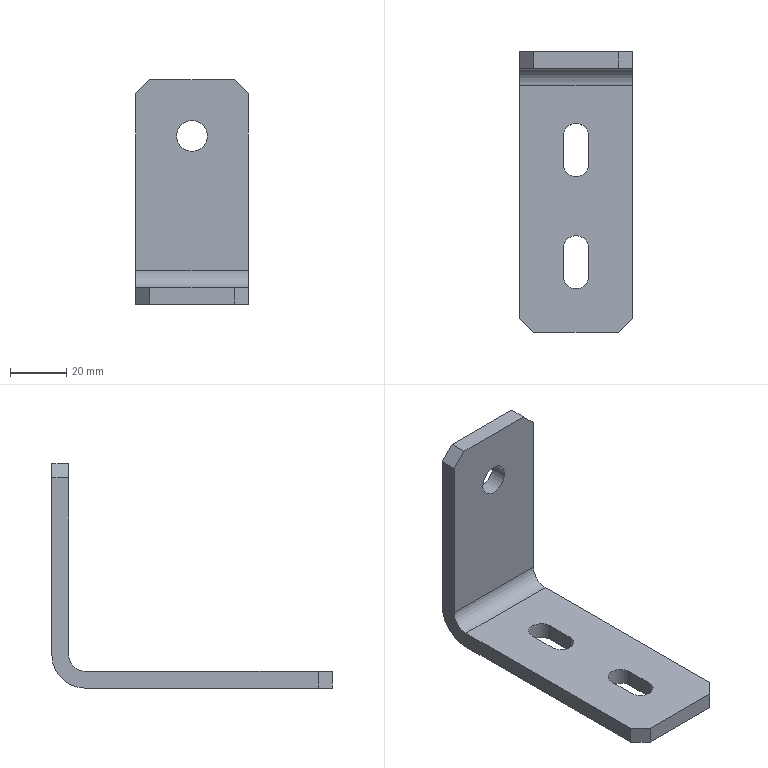Part | STEP file | support for guide | 1 solid | 23 faces | box 40 x 100 x 80 mm | volume 38119 mm3 | plane 16 | cylinder 6 | spline 1 | commonest cylinder face diameters 9 x4 12 x1 24 x1